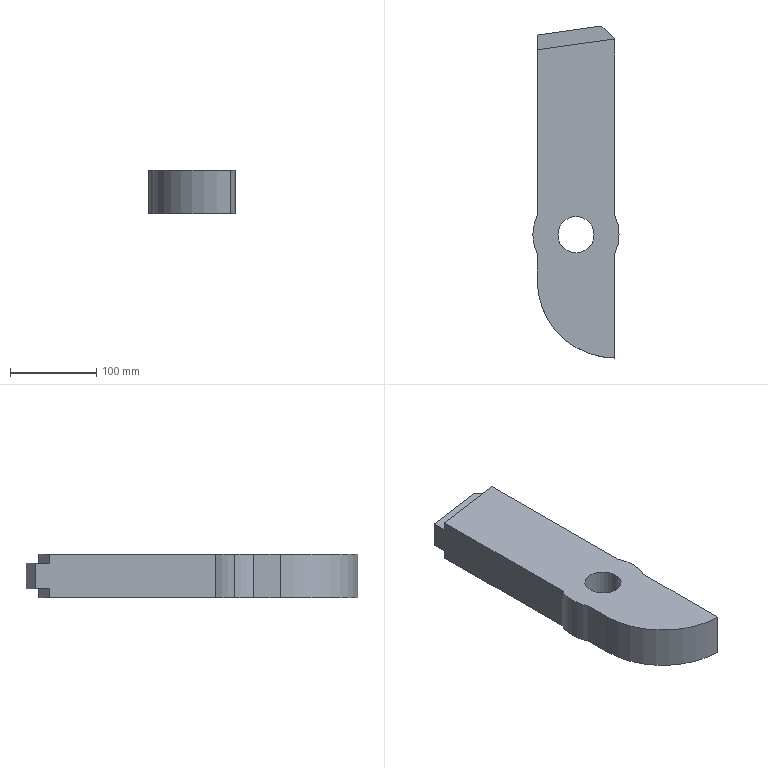Part | SolidWorks | features Extrusion 1, ICE 1 | 1 solid | 18 faces | box 100 x 385 x 50 mm | volume 1537454 mm3 | plane 12 | cylinder 6 | commonest cylinder face diameters 100 x3 42 x2 180 x1
STEP:
#1=CARTESIAN_POINT('',(-66.,143.,25.));
#2=VERTEX_POINT('',#1);
#3=CARTESIAN_POINT('',(-24.,143.,25.));
#4=VERTEX_POINT('',#3);
#5=CARTESIAN_POINT('',(-45.,143.,25.));
#6=DIRECTION('',(0.,0.,1.));
#7=DIRECTION('',(1.,0.,0.));
#8=AXIS2_PLACEMENT_3D('',#5,#6,#7);
#9=CIRCLE('',#8,21.);
#10=EDGE_CURVE('',#2,#4,#9,.T.);
#11=ORIENTED_EDGE('',*,*,#10,.T.);
#12=CARTESIAN_POINT('',(-24.,143.,-25.));
#13=VERTEX_POINT('',#12);
#14=CARTESIAN_POINT('',(-24.,143.,25.));
#15=DIRECTION('',(0.,0.,-1.));
#16=VECTOR('',#15,1000.);
#17=LINE('',#14,#16);
#18=EDGE_CURVE('',#4,#13,#17,.T.);
#19=ORIENTED_EDGE('',*,*,#18,.T.);
#20=CARTESIAN_POINT('',(-66.,143.,-25.));
#21=VERTEX_POINT('',#20);
#22=CARTESIAN_POINT('',(-45.,143.,-25.));
#23=DIRECTION('',(0.,0.,1.));
#24=DIRECTION('',(1.,0.,0.));
#25=AXIS2_PLACEMENT_3D('',#22,#23,#24);
#26=CIRCLE('',#25,21.);
#27=EDGE_CURVE('',#21,#13,#26,.T.);
#28=ORIENTED_EDGE('',*,*,#27,.F.);
#29=CARTESIAN_POINT('',(-66.,143.,25.));
#30=DIRECTION('',(0.,0.,-1.));
#31=VECTOR('',#30,1000.);
#32=LINE('',#29,#31);
#33=EDGE_CURVE('',#2,#21,#32,.T.);
#34=ORIENTED_EDGE('',*,*,#33,.F.);
#35=EDGE_LOOP('',(#11,#19,#28,#34));
#36=FACE_OUTER_BOUND('',#35,.T.);
#37=CARTESIAN_POINT('',(-45.,143.,25.));
#38=DIRECTION('',(0.,0.,-1.));
#39=DIRECTION('',(-1.,0.,0.));
#40=AXIS2_PLACEMENT_3D('',#37,#38,#39);
#41=CYLINDRICAL_SURFACE('',#40,21.);
#42=ADVANCED_FACE('',(#36),#41,.F.);
#43=CARTESIAN_POINT('',(-95.,143.,25.));
#44=VERTEX_POINT('',#43);
#45=CARTESIAN_POINT('',(-90.,121.206,25.));
#46=VERTEX_POINT('',#45);
#47=CARTESIAN_POINT('',(-45.,143.,25.));
#48=DIRECTION('',(0.,0.,1.));
#49=DIRECTION('',(1.,0.,0.));
#50=AXIS2_PLACEMENT_3D('',#47,#48,#49);
#51=CIRCLE('',#50,50.);
#52=EDGE_CURVE('',#44,#46,#51,.T.);
#53=ORIENTED_EDGE('',*,*,#52,.F.);
#54=CARTESIAN_POINT('',(-95.,143.,-25.));
#55=VERTEX_POINT('',#54);
#56=CARTESIAN_POINT('',(-95.,143.,25.));
#57=DIRECTION('',(0.,0.,-1.));
#58=VECTOR('',#57,1000.);
#59=LINE('',#56,#58);
#60=EDGE_CURVE('',#44,#55,#59,.T.);
#61=ORIENTED_EDGE('',*,*,#60,.T.);
#62=CARTESIAN_POINT('',(-90.,121.206,-25.));
#63=VERTEX_POINT('',#62);
#64=CARTESIAN_POINT('',(-45.,143.,-25.));
#65=DIRECTION('',(0.,0.,1.));
#66=DIRECTION('',(1.,0.,0.));
#67=AXIS2_PLACEMENT_3D('',#64,#65,#66);
#68=CIRCLE('',#67,50.);
#69=EDGE_CURVE('',#55,#63,#68,.T.);
#70=ORIENTED_EDGE('',*,*,#69,.T.);
#71=CARTESIAN_POINT('',(-90.,121.206,25.));
#72=DIRECTION('',(0.,0.,-1.));
#73=VECTOR('',#72,1000.);
#74=LINE('',#71,#73);
#75=EDGE_CURVE('',#46,#63,#74,.T.);
#76=ORIENTED_EDGE('',*,*,#75,.F.);
#77=EDGE_LOOP('',(#53,#61,#70,#76));
#78=FACE_OUTER_BOUND('',#77,.T.);
#79=CARTESIAN_POINT('',(-45.,143.,25.));
#80=DIRECTION('',(0.,0.,-1.));
#81=DIRECTION('',(-1.,0.,0.));
#82=AXIS2_PLACEMENT_3D('',#79,#80,#81);
#83=CYLINDRICAL_SURFACE('',#82,50.);
#84=ADVANCED_FACE('',(#78),#83,.T.);
#85=CARTESIAN_POINT('',(-15.,385.,-15.));
#86=VERTEX_POINT('',#85);
#87=CARTESIAN_POINT('',(-0.03685,370.037,-15.));
#88=VERTEX_POINT('',#87);
#89=CARTESIAN_POINT('',(0.,370.,-15.));
#90=DIRECTION('',(0.7071,-0.7071,0.));
#91=VECTOR('',#90,1000.);
#92=LINE('',#89,#91);
#93=EDGE_CURVE('',#86,#88,#92,.T.);
#94=ORIENTED_EDGE('',*,*,#93,.F.);
#95=CARTESIAN_POINT('',(-15.,385.,15.));
#96=VERTEX_POINT('',#95);
#97=CARTESIAN_POINT('',(-15.,385.,25.));
#98=DIRECTION('',(0.,0.,-1.));
#99=VECTOR('',#98,1000.);
#100=LINE('',#97,#99);
#101=EDGE_CURVE('',#96,#86,#100,.T.);
#102=ORIENTED_EDGE('',*,*,#101,.F.);
#103=CARTESIAN_POINT('',(-0.03685,370.037,15.));
#104=VERTEX_POINT('',#103);
#105=CARTESIAN_POINT('',(0.,370.,15.));
#106=DIRECTION('',(-0.7071,0.7071,0.));
#107=VECTOR('',#106,1000.);
#108=LINE('',#105,#107);
#109=EDGE_CURVE('',#104,#96,#108,.T.);
#110=ORIENTED_EDGE('',*,*,#109,.F.);
#111=CARTESIAN_POINT('',(-0.03685,370.037,25.));
#112=VERTEX_POINT('',#111);
#113=CARTESIAN_POINT('',(-0.03685,370.037,25.));
#114=DIRECTION('',(0.,0.,-1.));
#115=VECTOR('',#114,1000.);
#116=LINE('',#113,#115);
#117=EDGE_CURVE('',#112,#104,#116,.T.);
#118=ORIENTED_EDGE('',*,*,#117,.F.);
#119=CARTESIAN_POINT('',(0.,370.,25.));
#120=VERTEX_POINT('',#119);
#121=CARTESIAN_POINT('',(0.,370.,25.));
#122=DIRECTION('',(-0.7071,0.7071,0.));
#123=VECTOR('',#122,1000.);
#124=LINE('',#121,#123);
#125=EDGE_CURVE('',#120,#112,#124,.T.);
#126=ORIENTED_EDGE('',*,*,#125,.F.);
#127=CARTESIAN_POINT('',(0.,370.,-25.));
#128=VERTEX_POINT('',#127);
#129=CARTESIAN_POINT('',(0.,370.,25.));
#130=DIRECTION('',(0.,0.,-1.));
#131=VECTOR('',#130,1000.);
#132=LINE('',#129,#131);
#133=EDGE_CURVE('',#120,#128,#132,.T.);
#134=ORIENTED_EDGE('',*,*,#133,.T.);
#135=CARTESIAN_POINT('',(-0.03685,370.037,-25.));
#136=VERTEX_POINT('',#135);
#137=CARTESIAN_POINT('',(0.,370.,-25.));
#138=DIRECTION('',(-0.7071,0.7071,0.));
#139=VECTOR('',#138,1000.);
#140=LINE('',#137,#139);
#141=EDGE_CURVE('',#128,#136,#140,.T.);
#142=ORIENTED_EDGE('',*,*,#141,.T.);
#143=CARTESIAN_POINT('',(-0.03685,370.037,25.));
#144=DIRECTION('',(0.,0.,-1.));
#145=VECTOR('',#144,1000.);
#146=LINE('',#143,#145);
#147=EDGE_CURVE('',#88,#136,#146,.T.);
#148=ORIENTED_EDGE('',*,*,#147,.F.);
#149=EDGE_LOOP('',(#94,#102,#110,#118,#126,#134,#142,#148));
#150=FACE_OUTER_BOUND('',#149,.T.);
#151=CARTESIAN_POINT('',(0.,370.,25.));
#152=DIRECTION('',(-0.7071,-0.7071,0.));
#153=DIRECTION('',(0.7071,-0.7071,0.));
#154=AXIS2_PLACEMENT_3D('',#151,#152,#153);
#155=PLANE('',#154);
#156=ADVANCED_FACE('',(#150),#155,.F.);
#157=CARTESIAN_POINT('',(-90.,374.459,-15.));
#158=VERTEX_POINT('',#157);
#159=CARTESIAN_POINT('',(4.613,387.756,-15.));
#160=DIRECTION('',(-0.9903,-0.1392,0.));
#161=VECTOR('',#160,1000.);
#162=LINE('',#159,#161);
#163=EDGE_CURVE('',#86,#158,#162,.T.);
#164=ORIENTED_EDGE('',*,*,#163,.T.);
#165=CARTESIAN_POINT('',(-90.,374.459,15.));
#166=VERTEX_POINT('',#165);
#167=CARTESIAN_POINT('',(-90.,374.459,25.));
#168=DIRECTION('',(0.,0.,-1.));
#169=VECTOR('',#168,1000.);
#170=LINE('',#167,#169);
#171=EDGE_CURVE('',#166,#158,#170,.T.);
#172=ORIENTED_EDGE('',*,*,#171,.F.);
#173=CARTESIAN_POINT('',(4.613,387.756,15.));
#174=DIRECTION('',(-0.9903,-0.1392,0.));
#175=VECTOR('',#174,1000.);
#176=LINE('',#173,#175);
#177=EDGE_CURVE('',#96,#166,#176,.T.);
#178=ORIENTED_EDGE('',*,*,#177,.F.);
#179=ORIENTED_EDGE('',*,*,#101,.T.);
#180=EDGE_LOOP('',(#164,#172,#178,#179));
#181=FACE_OUTER_BOUND('',#180,.T.);
#182=CARTESIAN_POINT('',(-15.,385.,25.));
#183=DIRECTION('',(0.1392,-0.9903,0.));
#184=DIRECTION('',(0.9903,0.1392,0.));
#185=AXIS2_PLACEMENT_3D('',#182,#183,#184);
#186=PLANE('',#185);
#187=ADVANCED_FACE('',(#181),#186,.F.);
#188=CARTESIAN_POINT('',(-90.,357.393,-15.));
#189=VERTEX_POINT('',#188);
#190=CARTESIAN_POINT('',(-90.,374.459,-15.));
#191=DIRECTION('',(0.,1.,0.));
#192=VECTOR('',#191,1000.);
#193=LINE('',#190,#192);
#194=EDGE_CURVE('',#189,#158,#193,.T.);
#195=ORIENTED_EDGE('',*,*,#194,.F.);
#196=CARTESIAN_POINT('',(-90.,357.393,-25.));
#197=VERTEX_POINT('',#196);
#198=CARTESIAN_POINT('',(-90.,357.393,25.));
#199=DIRECTION('',(0.,0.,1.));
#200=VECTOR('',#199,1000.);
#201=LINE('',#198,#200);
#202=EDGE_CURVE('',#197,#189,#201,.T.);
#203=ORIENTED_EDGE('',*,*,#202,.F.);
#204=CARTESIAN_POINT('',(-90.,164.794,-25.));
#205=VERTEX_POINT('',#204);
#206=CARTESIAN_POINT('',(-90.,374.459,-25.));
#207=DIRECTION('',(0.,-1.,0.));
#208=VECTOR('',#207,1000.);
#209=LINE('',#206,#208);
#210=EDGE_CURVE('',#197,#205,#209,.T.);
#211=ORIENTED_EDGE('',*,*,#210,.T.);
#212=CARTESIAN_POINT('',(-90.,164.794,25.));
#213=VERTEX_POINT('',#212);
#214=CARTESIAN_POINT('',(-90.,164.794,25.));
#215=DIRECTION('',(0.,0.,-1.));
#216=VECTOR('',#215,1000.);
#217=LINE('',#214,#216);
#218=EDGE_CURVE('',#213,#205,#217,.T.);
#219=ORIENTED_EDGE('',*,*,#218,.F.);
#220=CARTESIAN_POINT('',(-90.,357.393,25.));
#221=VERTEX_POINT('',#220);
#222=CARTESIAN_POINT('',(-90.,374.459,25.));
#223=DIRECTION('',(0.,-1.,0.));
#224=VECTOR('',#223,1000.);
#225=LINE('',#222,#224);
#226=EDGE_CURVE('',#221,#213,#225,.T.);
#227=ORIENTED_EDGE('',*,*,#226,.F.);
#228=CARTESIAN_POINT('',(-90.,357.393,15.));
#229=VERTEX_POINT('',#228);
#230=CARTESIAN_POINT('',(-90.,357.393,25.));
#231=DIRECTION('',(0.,0.,1.));
#232=VECTOR('',#231,1000.);
#233=LINE('',#230,#232);
#234=EDGE_CURVE('',#229,#221,#233,.T.);
#235=ORIENTED_EDGE('',*,*,#234,.F.);
#236=CARTESIAN_POINT('',(-90.,374.459,15.));
#237=DIRECTION('',(0.,-1.,0.));
#238=VECTOR('',#237,1000.);
#239=LINE('',#236,#238);
#240=EDGE_CURVE('',#166,#229,#239,.T.);
#241=ORIENTED_EDGE('',*,*,#240,.F.);
#242=ORIENTED_EDGE('',*,*,#171,.T.);
#243=EDGE_LOOP('',(#195,#203,#211,#219,#227,#235,#241,#242));
#244=FACE_OUTER_BOUND('',#243,.T.);
#245=CARTESIAN_POINT('',(-90.,374.459,25.));
#246=DIRECTION('',(1.,0.,0.));
#247=DIRECTION('',(0.,1.,0.));
#248=AXIS2_PLACEMENT_3D('',#245,#246,#247);
#249=PLANE('',#248);
#250=ADVANCED_FACE('',(#244),#249,.F.);
#251=ORIENTED_EDGE('',*,*,#27,.T.);
#252=CARTESIAN_POINT('',(-45.,143.,-25.));
#253=DIRECTION('',(0.,0.,1.));
#254=DIRECTION('',(1.,0.,0.));
#255=AXIS2_PLACEMENT_3D('',#252,#253,#254);
#256=CIRCLE('',#255,21.);
#257=EDGE_CURVE('',#13,#21,#256,.T.);
#258=ORIENTED_EDGE('',*,*,#257,.T.);
#259=EDGE_LOOP('',(#251,#258));
#260=FACE_BOUND('',#259,.T.);
#261=CARTESIAN_POINT('',(-38.595,364.618,-25.));
#262=DIRECTION('',(-0.9903,-0.1392,0.));
#263=VECTOR('',#262,1000.);
#264=LINE('',#261,#263);
#265=EDGE_CURVE('',#136,#197,#264,.T.);
#266=ORIENTED_EDGE('',*,*,#265,.F.);
#267=ORIENTED_EDGE('',*,*,#141,.F.);
#268=CARTESIAN_POINT('',(0.,164.794,-25.));
#269=VERTEX_POINT('',#268);
#270=CARTESIAN_POINT('',(0.,164.794,-25.));
#271=DIRECTION('',(0.,1.,0.));
#272=VECTOR('',#271,1000.);
#273=LINE('',#270,#272);
#274=EDGE_CURVE('',#269,#128,#273,.T.);
#275=ORIENTED_EDGE('',*,*,#274,.F.);
#276=CARTESIAN_POINT('',(0.,121.206,-25.));
#277=VERTEX_POINT('',#276);
#278=CARTESIAN_POINT('',(-45.,143.,-25.));
#279=DIRECTION('',(0.,0.,1.));
#280=DIRECTION('',(1.,0.,0.));
#281=AXIS2_PLACEMENT_3D('',#278,#279,#280);
#282=CIRCLE('',#281,50.);
#283=EDGE_CURVE('',#277,#269,#282,.T.);
#284=ORIENTED_EDGE('',*,*,#283,.F.);
#285=CARTESIAN_POINT('',(0.,0.,-25.));
#286=VERTEX_POINT('',#285);
#287=CARTESIAN_POINT('',(0.,0.,-25.));
#288=DIRECTION('',(0.,1.,0.));
#289=VECTOR('',#288,1000.);
#290=LINE('',#287,#289);
#291=EDGE_CURVE('',#286,#277,#290,.T.);
#292=ORIENTED_EDGE('',*,*,#291,.F.);
#293=CARTESIAN_POINT('',(-90.,90.,-25.));
#294=VERTEX_POINT('',#293);
#295=CARTESIAN_POINT('',(0.,90.,-25.));
#296=DIRECTION('',(0.,0.,1.));
#297=DIRECTION('',(1.,0.,0.));
#298=AXIS2_PLACEMENT_3D('',#295,#296,#297);
#299=CIRCLE('',#298,90.);
#300=EDGE_CURVE('',#294,#286,#299,.T.);
#301=ORIENTED_EDGE('',*,*,#300,.F.);
#302=CARTESIAN_POINT('',(-90.,121.206,-25.));
#303=DIRECTION('',(0.,-1.,0.));
#304=VECTOR('',#303,1000.);
#305=LINE('',#302,#304);
#306=EDGE_CURVE('',#63,#294,#305,.T.);
#307=ORIENTED_EDGE('',*,*,#306,.F.);
#308=ORIENTED_EDGE('',*,*,#69,.F.);
#309=CARTESIAN_POINT('',(-45.,143.,-25.));
#310=DIRECTION('',(0.,0.,1.));
#311=DIRECTION('',(1.,0.,0.));
#312=AXIS2_PLACEMENT_3D('',#309,#310,#311);
#313=CIRCLE('',#312,50.);
#314=EDGE_CURVE('',#205,#55,#313,.T.);
#315=ORIENTED_EDGE('',*,*,#314,.F.);
#316=ORIENTED_EDGE('',*,*,#210,.F.);
#317=EDGE_LOOP('',(#266,#267,#275,#284,#292,#301,#307,#308,#315,#316));
#318=FACE_OUTER_BOUND('',#317,.T.);
#319=CARTESIAN_POINT('',(0.,90.,-25.));
#320=DIRECTION('',(0.,0.,1.));
#321=DIRECTION('',(1.,0.,0.));
#322=AXIS2_PLACEMENT_3D('',#319,#320,#321);
#323=PLANE('',#322);
#324=ADVANCED_FACE('',(#260,#318),#323,.F.);
#325=ORIENTED_EDGE('',*,*,#10,.F.);
#326=CARTESIAN_POINT('',(-45.,143.,25.));
#327=DIRECTION('',(0.,0.,1.));
#328=DIRECTION('',(1.,0.,0.));
#329=AXIS2_PLACEMENT_3D('',#326,#327,#328);
#330=CIRCLE('',#329,21.);
#331=EDGE_CURVE('',#4,#2,#330,.T.);
#332=ORIENTED_EDGE('',*,*,#331,.F.);
#333=EDGE_LOOP('',(#325,#332));
#334=FACE_BOUND('',#333,.T.);
#335=ORIENTED_EDGE('',*,*,#125,.T.);
#336=CARTESIAN_POINT('',(6.965,371.021,25.));
#337=DIRECTION('',(-0.9903,-0.1392,0.));
#338=VECTOR('',#337,1000.);
#339=LINE('',#336,#338);
#340=EDGE_CURVE('',#112,#221,#339,.T.);
#341=ORIENTED_EDGE('',*,*,#340,.T.);
#342=ORIENTED_EDGE('',*,*,#226,.T.);
#343=CARTESIAN_POINT('',(-45.,143.,25.));
#344=DIRECTION('',(0.,0.,1.));
#345=DIRECTION('',(1.,0.,0.));
#346=AXIS2_PLACEMENT_3D('',#343,#344,#345);
#347=CIRCLE('',#346,50.);
#348=EDGE_CURVE('',#213,#44,#347,.T.);
#349=ORIENTED_EDGE('',*,*,#348,.T.);
#350=ORIENTED_EDGE('',*,*,#52,.T.);
#351=CARTESIAN_POINT('',(-90.,90.,25.));
#352=VERTEX_POINT('',#351);
#353=CARTESIAN_POINT('',(-90.,121.206,25.));
#354=DIRECTION('',(0.,-1.,0.));
#355=VECTOR('',#354,1000.);
#356=LINE('',#353,#355);
#357=EDGE_CURVE('',#46,#352,#356,.T.);
#358=ORIENTED_EDGE('',*,*,#357,.T.);
#359=CARTESIAN_POINT('',(0.,0.,25.));
#360=VERTEX_POINT('',#359);
#361=CARTESIAN_POINT('',(0.,90.,25.));
#362=DIRECTION('',(0.,0.,1.));
#363=DIRECTION('',(1.,0.,0.));
#364=AXIS2_PLACEMENT_3D('',#361,#362,#363);
#365=CIRCLE('',#364,90.);
#366=EDGE_CURVE('',#352,#360,#365,.T.);
#367=ORIENTED_EDGE('',*,*,#366,.T.);
#368=CARTESIAN_POINT('',(0.,121.206,25.));
#369=VERTEX_POINT('',#368);
#370=CARTESIAN_POINT('',(0.,0.,25.));
#371=DIRECTION('',(0.,1.,0.));
#372=VECTOR('',#371,1000.);
#373=LINE('',#370,#372);
#374=EDGE_CURVE('',#360,#369,#373,.T.);
#375=ORIENTED_EDGE('',*,*,#374,.T.);
#376=CARTESIAN_POINT('',(0.,164.794,25.));
#377=VERTEX_POINT('',#376);
#378=CARTESIAN_POINT('',(-45.,143.,25.));
#379=DIRECTION('',(0.,0.,1.));
#380=DIRECTION('',(1.,0.,0.));
#381=AXIS2_PLACEMENT_3D('',#378,#379,#380);
#382=CIRCLE('',#381,50.);
#383=EDGE_CURVE('',#369,#377,#382,.T.);
#384=ORIENTED_EDGE('',*,*,#383,.T.);
#385=CARTESIAN_POINT('',(0.,164.794,25.));
#386=DIRECTION('',(0.,1.,0.));
#387=VECTOR('',#386,1000.);
#388=LINE('',#385,#387);
#389=EDGE_CURVE('',#377,#120,#388,.T.);
#390=ORIENTED_EDGE('',*,*,#389,.T.);
#391=EDGE_LOOP('',(#335,#341,#342,#349,#350,#358,#367,#375,#384,#390));
#392=FACE_OUTER_BOUND('',#391,.T.);
#393=CARTESIAN_POINT('',(0.,90.,25.));
#394=DIRECTION('',(0.,0.,1.));
#395=DIRECTION('',(1.,0.,0.));
#396=AXIS2_PLACEMENT_3D('',#393,#394,#395);
#397=PLANE('',#396);
#398=ADVANCED_FACE('',(#334,#392),#397,.T.);
#399=ORIENTED_EDGE('',*,*,#300,.T.);
#400=CARTESIAN_POINT('',(0.,0.,25.));
#401=DIRECTION('',(0.,0.,-1.));
#402=VECTOR('',#401,1000.);
#403=LINE('',#400,#402);
#404=EDGE_CURVE('',#360,#286,#403,.T.);
#405=ORIENTED_EDGE('',*,*,#404,.F.);
#406=ORIENTED_EDGE('',*,*,#366,.F.);
#407=CARTESIAN_POINT('',(-90.,90.,25.));
#408=DIRECTION('',(0.,0.,-1.));
#409=VECTOR('',#408,1000.);
#410=LINE('',#407,#409);
#411=EDGE_CURVE('',#352,#294,#410,.T.);
#412=ORIENTED_EDGE('',*,*,#411,.T.);
#413=EDGE_LOOP('',(#399,#405,#406,#412));
#414=FACE_OUTER_BOUND('',#413,.T.);
#415=CARTESIAN_POINT('',(0.,90.,25.));
#416=DIRECTION('',(0.,0.,-1.));
#417=DIRECTION('',(-1.,0.,0.));
#418=AXIS2_PLACEMENT_3D('',#415,#416,#417);
#419=CYLINDRICAL_SURFACE('',#418,90.);
#420=ADVANCED_FACE('',(#414),#419,.T.);
#421=ORIENTED_EDGE('',*,*,#291,.T.);
#422=CARTESIAN_POINT('',(0.,121.206,25.));
#423=DIRECTION('',(0.,0.,-1.));
#424=VECTOR('',#423,1000.);
#425=LINE('',#422,#424);
#426=EDGE_CURVE('',#369,#277,#425,.T.);
#427=ORIENTED_EDGE('',*,*,#426,.F.);
#428=ORIENTED_EDGE('',*,*,#374,.F.);
#429=ORIENTED_EDGE('',*,*,#404,.T.);
#430=EDGE_LOOP('',(#421,#427,#428,#429));
#431=FACE_OUTER_BOUND('',#430,.T.);
#432=CARTESIAN_POINT('',(0.,0.,25.));
#433=DIRECTION('',(-1.,0.,0.));
#434=DIRECTION('',(0.,0.,1.));
#435=AXIS2_PLACEMENT_3D('',#432,#433,#434);
#436=PLANE('',#435);
#437=ADVANCED_FACE('',(#431),#436,.F.);
#438=ORIENTED_EDGE('',*,*,#283,.T.);
#439=CARTESIAN_POINT('',(0.,164.794,25.));
#440=DIRECTION('',(0.,0.,-1.));
#441=VECTOR('',#440,1000.);
#442=LINE('',#439,#441);
#443=EDGE_CURVE('',#377,#269,#442,.T.);
#444=ORIENTED_EDGE('',*,*,#443,.F.);
#445=ORIENTED_EDGE('',*,*,#383,.F.);
#446=ORIENTED_EDGE('',*,*,#426,.T.);
#447=EDGE_LOOP('',(#438,#444,#445,#446));
#448=FACE_OUTER_BOUND('',#447,.T.);
#449=CARTESIAN_POINT('',(-45.,143.,25.));
#450=DIRECTION('',(0.,0.,-1.));
#451=DIRECTION('',(-1.,0.,0.));
#452=AXIS2_PLACEMENT_3D('',#449,#450,#451);
#453=CYLINDRICAL_SURFACE('',#452,50.);
#454=ADVANCED_FACE('',(#448),#453,.T.);
#455=ORIENTED_EDGE('',*,*,#274,.T.);
#456=ORIENTED_EDGE('',*,*,#133,.F.);
#457=ORIENTED_EDGE('',*,*,#389,.F.);
#458=ORIENTED_EDGE('',*,*,#443,.T.);
#459=EDGE_LOOP('',(#455,#456,#457,#458));
#460=FACE_OUTER_BOUND('',#459,.T.);
#461=CARTESIAN_POINT('',(0.,164.794,25.));
#462=DIRECTION('',(-1.,0.,0.));
#463=DIRECTION('',(0.,0.,1.));
#464=AXIS2_PLACEMENT_3D('',#461,#462,#463);
#465=PLANE('',#464);
#466=ADVANCED_FACE('',(#460),#465,.F.);
#467=ORIENTED_EDGE('',*,*,#60,.F.);
#468=ORIENTED_EDGE('',*,*,#348,.F.);
#469=ORIENTED_EDGE('',*,*,#218,.T.);
#470=ORIENTED_EDGE('',*,*,#314,.T.);
#471=EDGE_LOOP('',(#467,#468,#469,#470));
#472=FACE_OUTER_BOUND('',#471,.T.);
#473=CARTESIAN_POINT('',(-45.,143.,25.));
#474=DIRECTION('',(0.,0.,-1.));
#475=DIRECTION('',(-1.,0.,0.));
#476=AXIS2_PLACEMENT_3D('',#473,#474,#475);
#477=CYLINDRICAL_SURFACE('',#476,50.);
#478=ADVANCED_FACE('',(#472),#477,.T.);
#479=ORIENTED_EDGE('',*,*,#306,.T.);
#480=ORIENTED_EDGE('',*,*,#411,.F.);
#481=ORIENTED_EDGE('',*,*,#357,.F.);
#482=ORIENTED_EDGE('',*,*,#75,.T.);
#483=EDGE_LOOP('',(#479,#480,#481,#482));
#484=FACE_OUTER_BOUND('',#483,.T.);
#485=CARTESIAN_POINT('',(-90.,121.206,25.));
#486=DIRECTION('',(1.,0.,0.));
#487=DIRECTION('',(0.,0.,-1.));
#488=AXIS2_PLACEMENT_3D('',#485,#486,#487);
#489=PLANE('',#488);
#490=ADVANCED_FACE('',(#484),#489,.F.);
#491=ORIENTED_EDGE('',*,*,#18,.F.);
#492=ORIENTED_EDGE('',*,*,#331,.T.);
#493=ORIENTED_EDGE('',*,*,#33,.T.);
#494=ORIENTED_EDGE('',*,*,#257,.F.);
#495=EDGE_LOOP('',(#491,#492,#493,#494));
#496=FACE_OUTER_BOUND('',#495,.T.);
#497=CARTESIAN_POINT('',(-45.,143.,25.));
#498=DIRECTION('',(0.,0.,-1.));
#499=DIRECTION('',(-1.,0.,0.));
#500=AXIS2_PLACEMENT_3D('',#497,#498,#499);
#501=CYLINDRICAL_SURFACE('',#500,21.);
#502=ADVANCED_FACE('',(#496),#501,.F.);
#503=ORIENTED_EDGE('',*,*,#117,.T.);
#504=CARTESIAN_POINT('',(6.965,371.021,15.));
#505=DIRECTION('',(-0.9903,-0.1392,0.));
#506=VECTOR('',#505,1000.);
#507=LINE('',#504,#506);
#508=EDGE_CURVE('',#104,#229,#507,.T.);
#509=ORIENTED_EDGE('',*,*,#508,.T.);
#510=ORIENTED_EDGE('',*,*,#234,.T.);
#511=ORIENTED_EDGE('',*,*,#340,.F.);
#512=EDGE_LOOP('',(#503,#509,#510,#511));
#513=FACE_OUTER_BOUND('',#512,.T.);
#514=CARTESIAN_POINT('',(6.965,371.021,15.));
#515=DIRECTION('',(-0.1392,0.9903,0.));
#516=DIRECTION('',(-0.9903,-0.1392,0.));
#517=AXIS2_PLACEMENT_3D('',#514,#515,#516);
#518=PLANE('',#517);
#519=ADVANCED_FACE('',(#513),#518,.T.);
#520=ORIENTED_EDGE('',*,*,#109,.T.);
#521=ORIENTED_EDGE('',*,*,#177,.T.);
#522=ORIENTED_EDGE('',*,*,#240,.T.);
#523=ORIENTED_EDGE('',*,*,#508,.F.);
#524=EDGE_LOOP('',(#520,#521,#522,#523));
#525=FACE_OUTER_BOUND('',#524,.T.);
#526=CARTESIAN_POINT('',(4.613,387.756,15.));
#527=DIRECTION('',(0.,0.,1.));
#528=DIRECTION('',(0.,-1.,0.));
#529=AXIS2_PLACEMENT_3D('',#526,#527,#528);
#530=PLANE('',#529);
#531=ADVANCED_FACE('',(#525),#530,.T.);
#532=ORIENTED_EDGE('',*,*,#93,.T.);
#533=CARTESIAN_POINT('',(6.965,371.021,-15.));
#534=DIRECTION('',(-0.9903,-0.1392,0.));
#535=VECTOR('',#534,1000.);
#536=LINE('',#533,#535);
#537=EDGE_CURVE('',#88,#189,#536,.T.);
#538=ORIENTED_EDGE('',*,*,#537,.T.);
#539=ORIENTED_EDGE('',*,*,#194,.T.);
#540=ORIENTED_EDGE('',*,*,#163,.F.);
#541=EDGE_LOOP('',(#532,#538,#539,#540));
#542=FACE_OUTER_BOUND('',#541,.T.);
#543=CARTESIAN_POINT('',(4.613,387.756,-15.));
#544=DIRECTION('',(0.,0.,-1.));
#545=DIRECTION('',(0.,1.,0.));
#546=AXIS2_PLACEMENT_3D('',#543,#544,#545);
#547=PLANE('',#546);
#548=ADVANCED_FACE('',(#542),#547,.T.);
#549=ORIENTED_EDGE('',*,*,#147,.T.);
#550=ORIENTED_EDGE('',*,*,#265,.T.);
#551=ORIENTED_EDGE('',*,*,#202,.T.);
#552=ORIENTED_EDGE('',*,*,#537,.F.);
#553=EDGE_LOOP('',(#549,#550,#551,#552));
#554=FACE_OUTER_BOUND('',#553,.T.);
#555=CARTESIAN_POINT('',(6.965,371.021,-15.));
#556=DIRECTION('',(-0.1392,0.9903,0.));
#557=DIRECTION('',(-0.9903,-0.1392,0.));
#558=AXIS2_PLACEMENT_3D('',#555,#556,#557);
#559=PLANE('',#558);
#560=ADVANCED_FACE('',(#554),#559,.T.);
#561=CLOSED_SHELL('',(#42,#84,#156,#187,#250,#324,#398,#420,#437,#454,#466,#478,#490,#502,#519,#531,#548,#560));
#562=MANIFOLD_SOLID_BREP('',#561);
#563=CARTESIAN_POINT('',(0.,0.,0.));
#564=DIRECTION('',(0.,0.,1.));
#565=DIRECTION('',(1.,0.,0.));
#566=AXIS2_PLACEMENT_3D('',#563,#564,#565);
#567=(LENGTH_UNIT()NAMED_UNIT(*)SI_UNIT(.MILLI.,.METRE.));
#568=UNCERTAINTY_MEASURE_WITH_UNIT(LENGTH_MEASURE(0.00001),#567,'','');
#569=(NAMED_UNIT(*)PLANE_ANGLE_UNIT()SI_UNIT($,.RADIAN.));
#570=(NAMED_UNIT(*)SI_UNIT($,.STERADIAN.)SOLID_ANGLE_UNIT());
#571=(GEOMETRIC_REPRESENTATION_CONTEXT(3)GLOBAL_UNCERTAINTY_ASSIGNED_CONTEXT((#568))GLOBAL_UNIT_ASSIGNED_CONTEXT((#567,#569,#570))REPRESENTATION_CONTEXT('',''));
#572=ADVANCED_BREP_SHAPE_REPRESENTATION('',(#562,#566),#571);